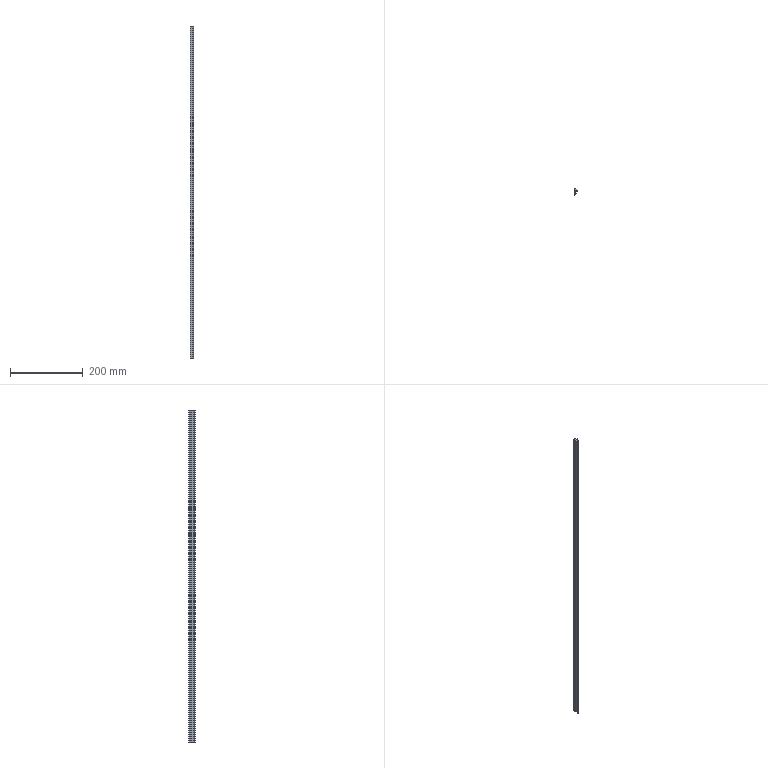Part | SolidWorks | features BaseBody 1, MoveFace 1 | 1 solid | 20 faces | box 10.8 x 17.5 x 914 mm | volume 72024 mm3 | cylinder 11 | plane 9 | commonest cylinder face diameters 1.6 x2 14 x2 0.4 x1 0.6 x1 0.8 x1 2.6 x1
STEP:
#1=CARTESIAN_POINT('',(-3.236,-11.055,814.));
#2=VERTEX_POINT('',#1);
#3=CARTESIAN_POINT('',(-4.3,-10.3,814.));
#4=VERTEX_POINT('',#3);
#5=CARTESIAN_POINT('',(-3.5,-10.3,814.));
#6=DIRECTION('',(0.,0.,-1.));
#7=DIRECTION('',(1.,0.,0.));
#8=AXIS2_PLACEMENT_3D('',#5,#6,#7);
#9=CIRCLE('',#8,0.8);
#10=EDGE_CURVE('',#2,#4,#9,.T.);
#11=ORIENTED_EDGE('',*,*,#10,.T.);
#12=CARTESIAN_POINT('',(-4.3,-10.3,-100.));
#13=VERTEX_POINT('',#12);
#14=CARTESIAN_POINT('',(-4.3,-10.3,-100.));
#15=DIRECTION('',(0.,0.,-1.));
#16=VECTOR('',#15,1000.);
#17=LINE('',#14,#16);
#18=EDGE_CURVE('',#4,#13,#17,.T.);
#19=ORIENTED_EDGE('',*,*,#18,.T.);
#20=CARTESIAN_POINT('',(-3.236,-11.055,-100.));
#21=VERTEX_POINT('',#20);
#22=CARTESIAN_POINT('',(-3.5,-10.3,-100.));
#23=DIRECTION('',(0.,0.,1.));
#24=DIRECTION('',(-1.,0.,0.));
#25=AXIS2_PLACEMENT_3D('',#22,#23,#24);
#26=CIRCLE('',#25,0.8);
#27=EDGE_CURVE('',#13,#21,#26,.T.);
#28=ORIENTED_EDGE('',*,*,#27,.T.);
#29=CARTESIAN_POINT('',(-3.236,-11.055,-100.));
#30=DIRECTION('',(0.,0.,-1.));
#31=VECTOR('',#30,1000.);
#32=LINE('',#29,#31);
#33=EDGE_CURVE('',#2,#21,#32,.T.);
#34=ORIENTED_EDGE('',*,*,#33,.F.);
#35=EDGE_LOOP('',(#11,#19,#28,#34));
#36=FACE_OUTER_BOUND('',#35,.T.);
#37=CARTESIAN_POINT('',(-3.5,-10.3,-100.));
#38=DIRECTION('',(0.,0.,-1.));
#39=DIRECTION('',(-1.,0.,0.));
#40=AXIS2_PLACEMENT_3D('',#37,#38,#39);
#41=CYLINDRICAL_SURFACE('',#40,0.8);
#42=ADVANCED_FACE('',(#36),#41,.T.);
#43=CARTESIAN_POINT('',(1.184,-6.397,-100.));
#44=VERTEX_POINT('',#43);
#45=CARTESIAN_POINT('',(-5.702,-4.29,-100.));
#46=DIRECTION('',(0.,0.,1.));
#47=DIRECTION('',(-1.,0.,0.));
#48=AXIS2_PLACEMENT_3D('',#45,#46,#47);
#49=CIRCLE('',#48,7.201);
#50=EDGE_CURVE('',#21,#44,#49,.T.);
#51=ORIENTED_EDGE('',*,*,#50,.T.);
#52=CARTESIAN_POINT('',(1.184,-6.397,814.));
#53=VERTEX_POINT('',#52);
#54=CARTESIAN_POINT('',(1.184,-6.397,-100.));
#55=DIRECTION('',(0.,0.,1.));
#56=VECTOR('',#55,1000.);
#57=LINE('',#54,#56);
#58=EDGE_CURVE('',#44,#53,#57,.T.);
#59=ORIENTED_EDGE('',*,*,#58,.T.);
#60=CARTESIAN_POINT('',(-5.702,-4.29,814.));
#61=DIRECTION('',(0.,0.,-1.));
#62=DIRECTION('',(1.,0.,0.));
#63=AXIS2_PLACEMENT_3D('',#60,#61,#62);
#64=CIRCLE('',#63,7.201);
#65=EDGE_CURVE('',#53,#2,#64,.T.);
#66=ORIENTED_EDGE('',*,*,#65,.T.);
#67=ORIENTED_EDGE('',*,*,#33,.T.);
#68=EDGE_LOOP('',(#51,#59,#66,#67));
#69=FACE_OUTER_BOUND('',#68,.T.);
#70=CARTESIAN_POINT('',(-5.702,-4.29,-100.));
#71=DIRECTION('',(0.,0.,-1.));
#72=DIRECTION('',(-1.,0.,0.));
#73=AXIS2_PLACEMENT_3D('',#70,#71,#72);
#74=CYLINDRICAL_SURFACE('',#73,7.201);
#75=ADVANCED_FACE('',(#69),#74,.T.);
#76=CARTESIAN_POINT('',(0.9,-6.,-100.));
#77=VERTEX_POINT('',#76);
#78=CARTESIAN_POINT('',(0.9,-6.3,-100.));
#79=DIRECTION('',(0.,0.,1.));
#80=DIRECTION('',(-1.,0.,0.));
#81=AXIS2_PLACEMENT_3D('',#78,#79,#80);
#82=CIRCLE('',#81,0.3);
#83=EDGE_CURVE('',#44,#77,#82,.T.);
#84=ORIENTED_EDGE('',*,*,#83,.T.);
#85=CARTESIAN_POINT('',(0.9,-6.,814.));
#86=VERTEX_POINT('',#85);
#87=CARTESIAN_POINT('',(0.9,-6.,-100.));
#88=DIRECTION('',(0.,0.,1.));
#89=VECTOR('',#88,1000.);
#90=LINE('',#87,#89);
#91=EDGE_CURVE('',#77,#86,#90,.T.);
#92=ORIENTED_EDGE('',*,*,#91,.T.);
#93=CARTESIAN_POINT('',(0.9,-6.3,814.));
#94=DIRECTION('',(0.,0.,-1.));
#95=DIRECTION('',(1.,0.,0.));
#96=AXIS2_PLACEMENT_3D('',#93,#94,#95);
#97=CIRCLE('',#96,0.3);
#98=EDGE_CURVE('',#86,#53,#97,.T.);
#99=ORIENTED_EDGE('',*,*,#98,.T.);
#100=ORIENTED_EDGE('',*,*,#58,.F.);
#101=EDGE_LOOP('',(#84,#92,#99,#100));
#102=FACE_OUTER_BOUND('',#101,.T.);
#103=CARTESIAN_POINT('',(0.9,-6.3,-100.));
#104=DIRECTION('',(0.,0.,-1.));
#105=DIRECTION('',(-1.,0.,0.));
#106=AXIS2_PLACEMENT_3D('',#103,#104,#105);
#107=CYLINDRICAL_SURFACE('',#106,0.3);
#108=ADVANCED_FACE('',(#102),#107,.T.);
#109=CARTESIAN_POINT('',(-2.5,-0.5,-100.));
#110=VERTEX_POINT('',#109);
#111=CARTESIAN_POINT('',(-2.5,-6.153,-100.));
#112=VERTEX_POINT('',#111);
#113=CARTESIAN_POINT('',(-2.5,-6.397,-100.));
#114=DIRECTION('',(0.,-1.,0.));
#115=VECTOR('',#114,1000.);
#116=LINE('',#113,#115);
#117=EDGE_CURVE('',#110,#112,#116,.T.);
#118=ORIENTED_EDGE('',*,*,#117,.F.);
#119=CARTESIAN_POINT('',(-4.2,1.695,-100.));
#120=VERTEX_POINT('',#119);
#121=CARTESIAN_POINT('',(-1.701,1.875,-100.));
#122=DIRECTION('',(0.,0.,1.));
#123=DIRECTION('',(-1.,0.,0.));
#124=AXIS2_PLACEMENT_3D('',#121,#122,#123);
#125=CIRCLE('',#124,2.506);
#126=EDGE_CURVE('',#120,#110,#125,.T.);
#127=ORIENTED_EDGE('',*,*,#126,.F.);
#128=CARTESIAN_POINT('',(-4.2,5.1,-100.));
#129=VERTEX_POINT('',#128);
#130=CARTESIAN_POINT('',(-4.2,-6.397,-100.));
#131=DIRECTION('',(0.,-1.,0.));
#132=VECTOR('',#131,1000.);
#133=LINE('',#130,#132);
#134=EDGE_CURVE('',#129,#120,#133,.T.);
#135=ORIENTED_EDGE('',*,*,#134,.F.);
#136=CARTESIAN_POINT('',(-2.892,6.4,-100.));
#137=VERTEX_POINT('',#136);
#138=CARTESIAN_POINT('',(-2.9,5.1,-100.));
#139=DIRECTION('',(0.,0.,1.));
#140=DIRECTION('',(-1.,0.,0.));
#141=AXIS2_PLACEMENT_3D('',#138,#139,#140);
#142=CIRCLE('',#141,1.3);
#143=EDGE_CURVE('',#137,#129,#142,.T.);
#144=ORIENTED_EDGE('',*,*,#143,.F.);
#145=CARTESIAN_POINT('',(0.5,5.5,-100.));
#146=VERTEX_POINT('',#145);
#147=CARTESIAN_POINT('',(-2.934,-0.5999,-100.));
#148=DIRECTION('',(0.,0.,1.));
#149=DIRECTION('',(-1.,0.,0.));
#150=AXIS2_PLACEMENT_3D('',#147,#148,#149);
#151=CIRCLE('',#150,7.);
#152=EDGE_CURVE('',#146,#137,#151,.T.);
#153=ORIENTED_EDGE('',*,*,#152,.F.);
#154=CARTESIAN_POINT('',(5.5,1.7,-100.));
#155=VERTEX_POINT('',#154);
#156=CARTESIAN_POINT('',(5.5,1.7,-100.));
#157=DIRECTION('',(-0.7962,0.6051,0.));
#158=VECTOR('',#157,1000.);
#159=LINE('',#156,#158);
#160=EDGE_CURVE('',#155,#146,#159,.T.);
#161=ORIENTED_EDGE('',*,*,#160,.F.);
#162=CARTESIAN_POINT('',(6.458,-0.2215,-100.));
#163=VERTEX_POINT('',#162);
#164=CARTESIAN_POINT('',(6.458,-0.2215,-100.));
#165=DIRECTION('',(-0.4462,0.8949,0.));
#166=VECTOR('',#165,1000.);
#167=LINE('',#164,#166);
#168=EDGE_CURVE('',#163,#155,#167,.T.);
#169=ORIENTED_EDGE('',*,*,#168,.F.);
#170=CARTESIAN_POINT('',(5.895,-0.7433,-100.));
#171=VERTEX_POINT('',#170);
#172=CARTESIAN_POINT('',(6.1,-0.4,-100.));
#173=DIRECTION('',(0.,0.,1.));
#174=DIRECTION('',(-1.,0.,0.));
#175=AXIS2_PLACEMENT_3D('',#172,#173,#174);
#176=CIRCLE('',#175,0.4);
#177=EDGE_CURVE('',#171,#163,#176,.T.);
#178=ORIENTED_EDGE('',*,*,#177,.F.);
#179=CARTESIAN_POINT('',(3.,0.,-100.));
#180=VERTEX_POINT('',#179);
#181=CARTESIAN_POINT('',(2.746,-6.995,-100.));
#182=DIRECTION('',(0.,0.,-1.));
#183=DIRECTION('',(-1.,0.,0.));
#184=AXIS2_PLACEMENT_3D('',#181,#182,#183);
#185=CIRCLE('',#184,7.);
#186=EDGE_CURVE('',#180,#171,#185,.T.);
#187=ORIENTED_EDGE('',*,*,#186,.F.);
#188=CARTESIAN_POINT('',(0.,0.,-100.));
#189=VERTEX_POINT('',#188);
#190=CARTESIAN_POINT('',(-6.814,0.,-100.));
#191=DIRECTION('',(1.,0.,0.));
#192=VECTOR('',#191,1000.);
#193=LINE('',#190,#192);
#194=EDGE_CURVE('',#189,#180,#193,.T.);
#195=ORIENTED_EDGE('',*,*,#194,.F.);
#196=CARTESIAN_POINT('',(0.,-5.8,-100.));
#197=VERTEX_POINT('',#196);
#198=CARTESIAN_POINT('',(0.,-6.397,-100.));
#199=DIRECTION('',(0.,1.,0.));
#200=VECTOR('',#199,1000.);
#201=LINE('',#198,#200);
#202=EDGE_CURVE('',#197,#189,#201,.T.);
#203=ORIENTED_EDGE('',*,*,#202,.F.);
#204=CARTESIAN_POINT('',(0.2,-6.,-100.));
#205=VERTEX_POINT('',#204);
#206=CARTESIAN_POINT('',(0.2,-5.8,-100.));
#207=DIRECTION('',(0.,0.,1.));
#208=DIRECTION('',(-1.,0.,0.));
#209=AXIS2_PLACEMENT_3D('',#206,#207,#208);
#210=CIRCLE('',#209,0.2);
#211=EDGE_CURVE('',#197,#205,#210,.T.);
#212=ORIENTED_EDGE('',*,*,#211,.T.);
#213=CARTESIAN_POINT('',(-6.814,-6.,-100.));
#214=DIRECTION('',(-1.,0.,0.));
#215=VECTOR('',#214,1000.);
#216=LINE('',#213,#215);
#217=EDGE_CURVE('',#77,#205,#216,.T.);
#218=ORIENTED_EDGE('',*,*,#217,.F.);
#219=ORIENTED_EDGE('',*,*,#83,.F.);
#220=ORIENTED_EDGE('',*,*,#50,.F.);
#221=ORIENTED_EDGE('',*,*,#27,.F.);
#222=CARTESIAN_POINT('',(-3.998,-9.674,-100.));
#223=VERTEX_POINT('',#222);
#224=CARTESIAN_POINT('',(-3.5,-10.3,-100.));
#225=DIRECTION('',(0.,0.,1.));
#226=DIRECTION('',(-1.,0.,0.));
#227=AXIS2_PLACEMENT_3D('',#224,#225,#226);
#228=CIRCLE('',#227,0.8);
#229=EDGE_CURVE('',#223,#13,#228,.T.);
#230=ORIENTED_EDGE('',*,*,#229,.F.);
#231=CARTESIAN_POINT('',(-6.814,-6.397,-100.));
#232=DIRECTION('',(0.,0.,-1.));
#233=DIRECTION('',(-1.,0.,0.));
#234=AXIS2_PLACEMENT_3D('',#231,#232,#233);
#235=CIRCLE('',#234,4.321);
#236=EDGE_CURVE('',#112,#223,#235,.T.);
#237=ORIENTED_EDGE('',*,*,#236,.F.);
#238=EDGE_LOOP('',(#118,#127,#135,#144,#153,#161,#169,#178,#187,#195,#203,#212,#218,#219,#220,#221,#230,#237));
#239=FACE_OUTER_BOUND('',#238,.T.);
#240=CARTESIAN_POINT('',(-6.814,-6.397,-100.));
#241=DIRECTION('',(0.,0.,1.));
#242=DIRECTION('',(1.,0.,0.));
#243=AXIS2_PLACEMENT_3D('',#240,#241,#242);
#244=PLANE('',#243);
#245=ADVANCED_FACE('',(#239),#244,.F.);
#246=ORIENTED_EDGE('',*,*,#18,.F.);
#247=CARTESIAN_POINT('',(-3.998,-9.674,814.));
#248=VERTEX_POINT('',#247);
#249=CARTESIAN_POINT('',(-3.5,-10.3,814.));
#250=DIRECTION('',(0.,0.,-1.));
#251=DIRECTION('',(1.,0.,0.));
#252=AXIS2_PLACEMENT_3D('',#249,#250,#251);
#253=CIRCLE('',#252,0.8);
#254=EDGE_CURVE('',#4,#248,#253,.T.);
#255=ORIENTED_EDGE('',*,*,#254,.T.);
#256=CARTESIAN_POINT('',(-3.998,-9.674,-100.));
#257=DIRECTION('',(0.,0.,-1.));
#258=VECTOR('',#257,1000.);
#259=LINE('',#256,#258);
#260=EDGE_CURVE('',#248,#223,#259,.T.);
#261=ORIENTED_EDGE('',*,*,#260,.T.);
#262=ORIENTED_EDGE('',*,*,#229,.T.);
#263=EDGE_LOOP('',(#246,#255,#261,#262));
#264=FACE_OUTER_BOUND('',#263,.T.);
#265=CARTESIAN_POINT('',(-3.5,-10.3,-100.));
#266=DIRECTION('',(0.,0.,-1.));
#267=DIRECTION('',(-1.,0.,0.));
#268=AXIS2_PLACEMENT_3D('',#265,#266,#267);
#269=CYLINDRICAL_SURFACE('',#268,0.8);
#270=ADVANCED_FACE('',(#264),#269,.T.);
#271=CARTESIAN_POINT('',(-4.2,1.695,814.));
#272=VERTEX_POINT('',#271);
#273=CARTESIAN_POINT('',(-2.5,-0.5,814.));
#274=VERTEX_POINT('',#273);
#275=CARTESIAN_POINT('',(-1.701,1.875,814.));
#276=DIRECTION('',(0.,0.,1.));
#277=DIRECTION('',(1.,0.,0.));
#278=AXIS2_PLACEMENT_3D('',#275,#276,#277);
#279=CIRCLE('',#278,2.506);
#280=EDGE_CURVE('',#272,#274,#279,.T.);
#281=ORIENTED_EDGE('',*,*,#280,.T.);
#282=CARTESIAN_POINT('',(-2.5,-6.153,814.));
#283=VERTEX_POINT('',#282);
#284=CARTESIAN_POINT('',(-2.5,-6.397,814.));
#285=DIRECTION('',(0.,-1.,0.));
#286=VECTOR('',#285,1000.);
#287=LINE('',#284,#286);
#288=EDGE_CURVE('',#274,#283,#287,.T.);
#289=ORIENTED_EDGE('',*,*,#288,.T.);
#290=CARTESIAN_POINT('',(-6.814,-6.397,814.));
#291=DIRECTION('',(0.,0.,-1.));
#292=DIRECTION('',(1.,0.,0.));
#293=AXIS2_PLACEMENT_3D('',#290,#291,#292);
#294=CIRCLE('',#293,4.321);
#295=EDGE_CURVE('',#283,#248,#294,.T.);
#296=ORIENTED_EDGE('',*,*,#295,.T.);
#297=ORIENTED_EDGE('',*,*,#254,.F.);
#298=ORIENTED_EDGE('',*,*,#10,.F.);
#299=ORIENTED_EDGE('',*,*,#65,.F.);
#300=ORIENTED_EDGE('',*,*,#98,.F.);
#301=CARTESIAN_POINT('',(0.2,-6.,814.));
#302=VERTEX_POINT('',#301);
#303=CARTESIAN_POINT('',(-6.814,-6.,814.));
#304=DIRECTION('',(-1.,0.,0.));
#305=VECTOR('',#304,1000.);
#306=LINE('',#303,#305);
#307=EDGE_CURVE('',#86,#302,#306,.T.);
#308=ORIENTED_EDGE('',*,*,#307,.T.);
#309=CARTESIAN_POINT('',(0.,-5.8,814.));
#310=VERTEX_POINT('',#309);
#311=CARTESIAN_POINT('',(0.2,-5.8,814.));
#312=DIRECTION('',(0.,0.,-1.));
#313=DIRECTION('',(1.,0.,0.));
#314=AXIS2_PLACEMENT_3D('',#311,#312,#313);
#315=CIRCLE('',#314,0.2);
#316=EDGE_CURVE('',#302,#310,#315,.T.);
#317=ORIENTED_EDGE('',*,*,#316,.T.);
#318=CARTESIAN_POINT('',(0.,0.,814.));
#319=VERTEX_POINT('',#318);
#320=CARTESIAN_POINT('',(0.,-6.397,814.));
#321=DIRECTION('',(0.,1.,0.));
#322=VECTOR('',#321,1000.);
#323=LINE('',#320,#322);
#324=EDGE_CURVE('',#310,#319,#323,.T.);
#325=ORIENTED_EDGE('',*,*,#324,.T.);
#326=CARTESIAN_POINT('',(3.,0.,814.));
#327=VERTEX_POINT('',#326);
#328=CARTESIAN_POINT('',(-6.814,0.,814.));
#329=DIRECTION('',(1.,0.,0.));
#330=VECTOR('',#329,1000.);
#331=LINE('',#328,#330);
#332=EDGE_CURVE('',#319,#327,#331,.T.);
#333=ORIENTED_EDGE('',*,*,#332,.T.);
#334=CARTESIAN_POINT('',(5.895,-0.7433,814.));
#335=VERTEX_POINT('',#334);
#336=CARTESIAN_POINT('',(2.746,-6.995,814.));
#337=DIRECTION('',(0.,0.,-1.));
#338=DIRECTION('',(1.,0.,0.));
#339=AXIS2_PLACEMENT_3D('',#336,#337,#338);
#340=CIRCLE('',#339,7.);
#341=EDGE_CURVE('',#327,#335,#340,.T.);
#342=ORIENTED_EDGE('',*,*,#341,.T.);
#343=CARTESIAN_POINT('',(6.458,-0.2215,814.));
#344=VERTEX_POINT('',#343);
#345=CARTESIAN_POINT('',(6.1,-0.4,814.));
#346=DIRECTION('',(0.,0.,-1.));
#347=DIRECTION('',(1.,0.,0.));
#348=AXIS2_PLACEMENT_3D('',#345,#346,#347);
#349=CIRCLE('',#348,0.4);
#350=EDGE_CURVE('',#344,#335,#349,.T.);
#351=ORIENTED_EDGE('',*,*,#350,.F.);
#352=CARTESIAN_POINT('',(5.5,1.7,814.));
#353=VERTEX_POINT('',#352);
#354=CARTESIAN_POINT('',(6.282,0.1323,814.));
#355=DIRECTION('',(-0.4462,0.8949,0.));
#356=VECTOR('',#355,1000.);
#357=LINE('',#354,#356);
#358=EDGE_CURVE('',#344,#353,#357,.T.);
#359=ORIENTED_EDGE('',*,*,#358,.T.);
#360=CARTESIAN_POINT('',(0.5,5.5,814.));
#361=VERTEX_POINT('',#360);
#362=CARTESIAN_POINT('',(1.595,4.668,814.));
#363=DIRECTION('',(-0.7962,0.6051,0.));
#364=VECTOR('',#363,1000.);
#365=LINE('',#362,#364);
#366=EDGE_CURVE('',#353,#361,#365,.T.);
#367=ORIENTED_EDGE('',*,*,#366,.T.);
#368=CARTESIAN_POINT('',(-2.892,6.4,814.));
#369=VERTEX_POINT('',#368);
#370=CARTESIAN_POINT('',(-2.934,-0.5999,814.));
#371=DIRECTION('',(0.,0.,1.));
#372=DIRECTION('',(1.,0.,0.));
#373=AXIS2_PLACEMENT_3D('',#370,#371,#372);
#374=CIRCLE('',#373,7.);
#375=EDGE_CURVE('',#361,#369,#374,.T.);
#376=ORIENTED_EDGE('',*,*,#375,.T.);
#377=CARTESIAN_POINT('',(-4.2,5.1,814.));
#378=VERTEX_POINT('',#377);
#379=CARTESIAN_POINT('',(-2.9,5.1,814.));
#380=DIRECTION('',(0.,0.,1.));
#381=DIRECTION('',(1.,0.,0.));
#382=AXIS2_PLACEMENT_3D('',#379,#380,#381);
#383=CIRCLE('',#382,1.3);
#384=EDGE_CURVE('',#369,#378,#383,.T.);
#385=ORIENTED_EDGE('',*,*,#384,.T.);
#386=CARTESIAN_POINT('',(-4.2,-6.397,814.));
#387=DIRECTION('',(0.,-1.,0.));
#388=VECTOR('',#387,1000.);
#389=LINE('',#386,#388);
#390=EDGE_CURVE('',#378,#272,#389,.T.);
#391=ORIENTED_EDGE('',*,*,#390,.T.);
#392=EDGE_LOOP('',(#281,#289,#296,#297,#298,#299,#300,#308,#317,#325,#333,#342,#351,#359,#367,#376,#385,#391));
#393=FACE_OUTER_BOUND('',#392,.T.);
#394=CARTESIAN_POINT('',(-6.814,-6.397,814.));
#395=DIRECTION('',(0.,0.,1.));
#396=DIRECTION('',(1.,0.,0.));
#397=AXIS2_PLACEMENT_3D('',#394,#395,#396);
#398=PLANE('',#397);
#399=ADVANCED_FACE('',(#393),#398,.T.);
#400=ORIENTED_EDGE('',*,*,#217,.T.);
#401=CARTESIAN_POINT('',(0.2,-6.,-100.));
#402=DIRECTION('',(0.,0.,1.));
#403=VECTOR('',#402,1000.);
#404=LINE('',#401,#403);
#405=EDGE_CURVE('',#205,#302,#404,.T.);
#406=ORIENTED_EDGE('',*,*,#405,.T.);
#407=ORIENTED_EDGE('',*,*,#307,.F.);
#408=ORIENTED_EDGE('',*,*,#91,.F.);
#409=EDGE_LOOP('',(#400,#406,#407,#408));
#410=FACE_OUTER_BOUND('',#409,.T.);
#411=CARTESIAN_POINT('',(0.9,-6.,-100.));
#412=DIRECTION('',(0.,1.,0.));
#413=DIRECTION('',(0.,0.,1.));
#414=AXIS2_PLACEMENT_3D('',#411,#412,#413);
#415=PLANE('',#414);
#416=ADVANCED_FACE('',(#410),#415,.T.);
#417=CARTESIAN_POINT('',(-2.5,-6.153,-100.));
#418=DIRECTION('',(0.,0.,1.));
#419=VECTOR('',#418,1000.);
#420=LINE('',#417,#419);
#421=EDGE_CURVE('',#112,#283,#420,.T.);
#422=ORIENTED_EDGE('',*,*,#421,.F.);
#423=ORIENTED_EDGE('',*,*,#236,.T.);
#424=ORIENTED_EDGE('',*,*,#260,.F.);
#425=ORIENTED_EDGE('',*,*,#295,.F.);
#426=EDGE_LOOP('',(#422,#423,#424,#425));
#427=FACE_OUTER_BOUND('',#426,.T.);
#428=CARTESIAN_POINT('',(-6.814,-6.397,-100.));
#429=DIRECTION('',(0.,0.,-1.));
#430=DIRECTION('',(-1.,0.,0.));
#431=AXIS2_PLACEMENT_3D('',#428,#429,#430);
#432=CYLINDRICAL_SURFACE('',#431,4.321);
#433=ADVANCED_FACE('',(#427),#432,.F.);
#434=ORIENTED_EDGE('',*,*,#117,.T.);
#435=ORIENTED_EDGE('',*,*,#421,.T.);
#436=ORIENTED_EDGE('',*,*,#288,.F.);
#437=CARTESIAN_POINT('',(-2.5,-0.5,-100.));
#438=DIRECTION('',(0.,0.,-1.));
#439=VECTOR('',#438,1000.);
#440=LINE('',#437,#439);
#441=EDGE_CURVE('',#274,#110,#440,.T.);
#442=ORIENTED_EDGE('',*,*,#441,.T.);
#443=EDGE_LOOP('',(#434,#435,#436,#442));
#444=FACE_OUTER_BOUND('',#443,.T.);
#445=CARTESIAN_POINT('',(-2.5,-0.5,-100.));
#446=DIRECTION('',(-1.,0.,0.));
#447=DIRECTION('',(0.,0.,1.));
#448=AXIS2_PLACEMENT_3D('',#445,#446,#447);
#449=PLANE('',#448);
#450=ADVANCED_FACE('',(#444),#449,.T.);
#451=ORIENTED_EDGE('',*,*,#126,.T.);
#452=ORIENTED_EDGE('',*,*,#441,.F.);
#453=ORIENTED_EDGE('',*,*,#280,.F.);
#454=CARTESIAN_POINT('',(-4.2,1.695,-100.));
#455=DIRECTION('',(0.,0.,-1.));
#456=VECTOR('',#455,1000.);
#457=LINE('',#454,#456);
#458=EDGE_CURVE('',#272,#120,#457,.T.);
#459=ORIENTED_EDGE('',*,*,#458,.T.);
#460=EDGE_LOOP('',(#451,#452,#453,#459));
#461=FACE_OUTER_BOUND('',#460,.T.);
#462=CARTESIAN_POINT('',(-1.701,1.875,-100.));
#463=DIRECTION('',(0.,0.,-1.));
#464=DIRECTION('',(-1.,0.,0.));
#465=AXIS2_PLACEMENT_3D('',#462,#463,#464);
#466=CYLINDRICAL_SURFACE('',#465,2.506);
#467=ADVANCED_FACE('',(#461),#466,.T.);
#468=ORIENTED_EDGE('',*,*,#134,.T.);
#469=ORIENTED_EDGE('',*,*,#458,.F.);
#470=ORIENTED_EDGE('',*,*,#390,.F.);
#471=CARTESIAN_POINT('',(-4.2,5.1,-100.));
#472=DIRECTION('',(0.,0.,-1.));
#473=VECTOR('',#472,1000.);
#474=LINE('',#471,#473);
#475=EDGE_CURVE('',#378,#129,#474,.T.);
#476=ORIENTED_EDGE('',*,*,#475,.T.);
#477=EDGE_LOOP('',(#468,#469,#470,#476));
#478=FACE_OUTER_BOUND('',#477,.T.);
#479=CARTESIAN_POINT('',(-4.2,5.1,-100.));
#480=DIRECTION('',(-1.,0.,0.));
#481=DIRECTION('',(0.,0.,1.));
#482=AXIS2_PLACEMENT_3D('',#479,#480,#481);
#483=PLANE('',#482);
#484=ADVANCED_FACE('',(#478),#483,.T.);
#485=ORIENTED_EDGE('',*,*,#143,.T.);
#486=ORIENTED_EDGE('',*,*,#475,.F.);
#487=ORIENTED_EDGE('',*,*,#384,.F.);
#488=CARTESIAN_POINT('',(-2.892,6.4,-100.));
#489=DIRECTION('',(0.,0.,-1.));
#490=VECTOR('',#489,1000.);
#491=LINE('',#488,#490);
#492=EDGE_CURVE('',#369,#137,#491,.T.);
#493=ORIENTED_EDGE('',*,*,#492,.T.);
#494=EDGE_LOOP('',(#485,#486,#487,#493));
#495=FACE_OUTER_BOUND('',#494,.T.);
#496=CARTESIAN_POINT('',(-2.9,5.1,-100.));
#497=DIRECTION('',(0.,0.,-1.));
#498=DIRECTION('',(-1.,0.,0.));
#499=AXIS2_PLACEMENT_3D('',#496,#497,#498);
#500=CYLINDRICAL_SURFACE('',#499,1.3);
#501=ADVANCED_FACE('',(#495),#500,.T.);
#502=ORIENTED_EDGE('',*,*,#152,.T.);
#503=ORIENTED_EDGE('',*,*,#492,.F.);
#504=ORIENTED_EDGE('',*,*,#375,.F.);
#505=CARTESIAN_POINT('',(0.5,5.5,-100.));
#506=DIRECTION('',(0.,0.,-1.));
#507=VECTOR('',#506,1000.);
#508=LINE('',#505,#507);
#509=EDGE_CURVE('',#361,#146,#508,.T.);
#510=ORIENTED_EDGE('',*,*,#509,.T.);
#511=EDGE_LOOP('',(#502,#503,#504,#510));
#512=FACE_OUTER_BOUND('',#511,.T.);
#513=CARTESIAN_POINT('',(-2.934,-0.5999,-100.));
#514=DIRECTION('',(0.,0.,-1.));
#515=DIRECTION('',(-1.,0.,0.));
#516=AXIS2_PLACEMENT_3D('',#513,#514,#515);
#517=CYLINDRICAL_SURFACE('',#516,7.);
#518=ADVANCED_FACE('',(#512),#517,.T.);
#519=ORIENTED_EDGE('',*,*,#160,.T.);
#520=ORIENTED_EDGE('',*,*,#509,.F.);
#521=ORIENTED_EDGE('',*,*,#366,.F.);
#522=CARTESIAN_POINT('',(5.5,1.7,-100.));
#523=DIRECTION('',(0.,0.,-1.));
#524=VECTOR('',#523,1000.);
#525=LINE('',#522,#524);
#526=EDGE_CURVE('',#353,#155,#525,.T.);
#527=ORIENTED_EDGE('',*,*,#526,.T.);
#528=EDGE_LOOP('',(#519,#520,#521,#527));
#529=FACE_OUTER_BOUND('',#528,.T.);
#530=CARTESIAN_POINT('',(5.5,1.7,-100.));
#531=DIRECTION('',(0.6051,0.7962,0.));
#532=DIRECTION('',(-0.7962,0.6051,0.));
#533=AXIS2_PLACEMENT_3D('',#530,#531,#532);
#534=PLANE('',#533);
#535=ADVANCED_FACE('',(#529),#534,.T.);
#536=ORIENTED_EDGE('',*,*,#168,.T.);
#537=ORIENTED_EDGE('',*,*,#526,.F.);
#538=ORIENTED_EDGE('',*,*,#358,.F.);
#539=CARTESIAN_POINT('',(6.458,-0.2215,-100.));
#540=DIRECTION('',(0.,0.,-1.));
#541=VECTOR('',#540,1000.);
#542=LINE('',#539,#541);
#543=EDGE_CURVE('',#344,#163,#542,.T.);
#544=ORIENTED_EDGE('',*,*,#543,.T.);
#545=EDGE_LOOP('',(#536,#537,#538,#544));
#546=FACE_OUTER_BOUND('',#545,.T.);
#547=CARTESIAN_POINT('',(6.458,-0.2215,-100.));
#548=DIRECTION('',(0.8949,0.4462,0.));
#549=DIRECTION('',(-0.4462,0.8949,0.));
#550=AXIS2_PLACEMENT_3D('',#547,#548,#549);
#551=PLANE('',#550);
#552=ADVANCED_FACE('',(#546),#551,.T.);
#553=CARTESIAN_POINT('',(3.,0.,-100.));
#554=DIRECTION('',(0.,0.,1.));
#555=VECTOR('',#554,1000.);
#556=LINE('',#553,#555);
#557=EDGE_CURVE('',#180,#327,#556,.T.);
#558=ORIENTED_EDGE('',*,*,#557,.F.);
#559=ORIENTED_EDGE('',*,*,#186,.T.);
#560=CARTESIAN_POINT('',(5.895,-0.7433,-100.));
#561=DIRECTION('',(0.,0.,-1.));
#562=VECTOR('',#561,1000.);
#563=LINE('',#560,#562);
#564=EDGE_CURVE('',#335,#171,#563,.T.);
#565=ORIENTED_EDGE('',*,*,#564,.F.);
#566=ORIENTED_EDGE('',*,*,#341,.F.);
#567=EDGE_LOOP('',(#558,#559,#565,#566));
#568=FACE_OUTER_BOUND('',#567,.T.);
#569=CARTESIAN_POINT('',(2.746,-6.995,-100.));
#570=DIRECTION('',(0.,0.,-1.));
#571=DIRECTION('',(-1.,0.,0.));
#572=AXIS2_PLACEMENT_3D('',#569,#570,#571);
#573=CYLINDRICAL_SURFACE('',#572,7.);
#574=ADVANCED_FACE('',(#568),#573,.F.);
#575=ORIENTED_EDGE('',*,*,#194,.T.);
#576=ORIENTED_EDGE('',*,*,#557,.T.);
#577=ORIENTED_EDGE('',*,*,#332,.F.);
#578=CARTESIAN_POINT('',(0.,0.,-100.));
#579=DIRECTION('',(0.,0.,-1.));
#580=VECTOR('',#579,1000.);
#581=LINE('',#578,#580);
#582=EDGE_CURVE('',#319,#189,#581,.T.);
#583=ORIENTED_EDGE('',*,*,#582,.T.);
#584=EDGE_LOOP('',(#575,#576,#577,#583));
#585=FACE_OUTER_BOUND('',#584,.T.);
#586=CARTESIAN_POINT('',(0.,0.,-100.));
#587=DIRECTION('',(0.,-1.,0.));
#588=DIRECTION('',(0.,0.,-1.));
#589=AXIS2_PLACEMENT_3D('',#586,#587,#588);
#590=PLANE('',#589);
#591=ADVANCED_FACE('',(#585),#590,.T.);
#592=ORIENTED_EDGE('',*,*,#202,.T.);
#593=ORIENTED_EDGE('',*,*,#582,.F.);
#594=ORIENTED_EDGE('',*,*,#324,.F.);
#595=CARTESIAN_POINT('',(0.,-5.8,-100.));
#596=DIRECTION('',(0.,0.,-1.));
#597=VECTOR('',#596,1000.);
#598=LINE('',#595,#597);
#599=EDGE_CURVE('',#310,#197,#598,.T.);
#600=ORIENTED_EDGE('',*,*,#599,.T.);
#601=EDGE_LOOP('',(#592,#593,#594,#600));
#602=FACE_OUTER_BOUND('',#601,.T.);
#603=CARTESIAN_POINT('',(0.,-5.8,-100.));
#604=DIRECTION('',(1.,0.,0.));
#605=DIRECTION('',(0.,0.,-1.));
#606=AXIS2_PLACEMENT_3D('',#603,#604,#605);
#607=PLANE('',#606);
#608=ADVANCED_FACE('',(#602),#607,.T.);
#609=ORIENTED_EDGE('',*,*,#405,.F.);
#610=ORIENTED_EDGE('',*,*,#211,.F.);
#611=ORIENTED_EDGE('',*,*,#599,.F.);
#612=ORIENTED_EDGE('',*,*,#316,.F.);
#613=EDGE_LOOP('',(#609,#610,#611,#612));
#614=FACE_OUTER_BOUND('',#613,.T.);
#615=CARTESIAN_POINT('',(0.2,-5.8,-100.));
#616=DIRECTION('',(0.,0.,-1.));
#617=DIRECTION('',(-1.,0.,0.));
#618=AXIS2_PLACEMENT_3D('',#615,#616,#617);
#619=CYLINDRICAL_SURFACE('',#618,0.2);
#620=ADVANCED_FACE('',(#614),#619,.F.);
#621=ORIENTED_EDGE('',*,*,#177,.T.);
#622=ORIENTED_EDGE('',*,*,#543,.F.);
#623=ORIENTED_EDGE('',*,*,#350,.T.);
#624=ORIENTED_EDGE('',*,*,#564,.T.);
#625=EDGE_LOOP('',(#621,#622,#623,#624));
#626=FACE_OUTER_BOUND('',#625,.T.);
#627=CARTESIAN_POINT('',(6.1,-0.4,-100.));
#628=DIRECTION('',(0.,0.,-1.));
#629=DIRECTION('',(-1.,0.,0.));
#630=AXIS2_PLACEMENT_3D('',#627,#628,#629);
#631=CYLINDRICAL_SURFACE('',#630,0.4);
#632=ADVANCED_FACE('',(#626),#631,.T.);
#633=CLOSED_SHELL('',(#42,#75,#108,#245,#270,#399,#416,#433,#450,#467,#484,#501,#518,#535,#552,#574,#591,#608,#620,#632));
#634=MANIFOLD_SOLID_BREP('',#633);
#635=CARTESIAN_POINT('',(0.,0.,0.));
#636=DIRECTION('',(0.,0.,1.));
#637=DIRECTION('',(1.,0.,0.));
#638=AXIS2_PLACEMENT_3D('',#635,#636,#637);
#639=(LENGTH_UNIT()NAMED_UNIT(*)SI_UNIT(.MILLI.,.METRE.));
#640=UNCERTAINTY_MEASURE_WITH_UNIT(LENGTH_MEASURE(0.00001),#639,'','');
#641=(NAMED_UNIT(*)PLANE_ANGLE_UNIT()SI_UNIT($,.RADIAN.));
#642=(NAMED_UNIT(*)SI_UNIT($,.STERADIAN.)SOLID_ANGLE_UNIT());
#643=(GEOMETRIC_REPRESENTATION_CONTEXT(3)GLOBAL_UNCERTAINTY_ASSIGNED_CONTEXT((#640))GLOBAL_UNIT_ASSIGNED_CONTEXT((#639,#641,#642))REPRESENTATION_CONTEXT('',''));
#644=ADVANCED_BREP_SHAPE_REPRESENTATION('',(#634,#638),#643);